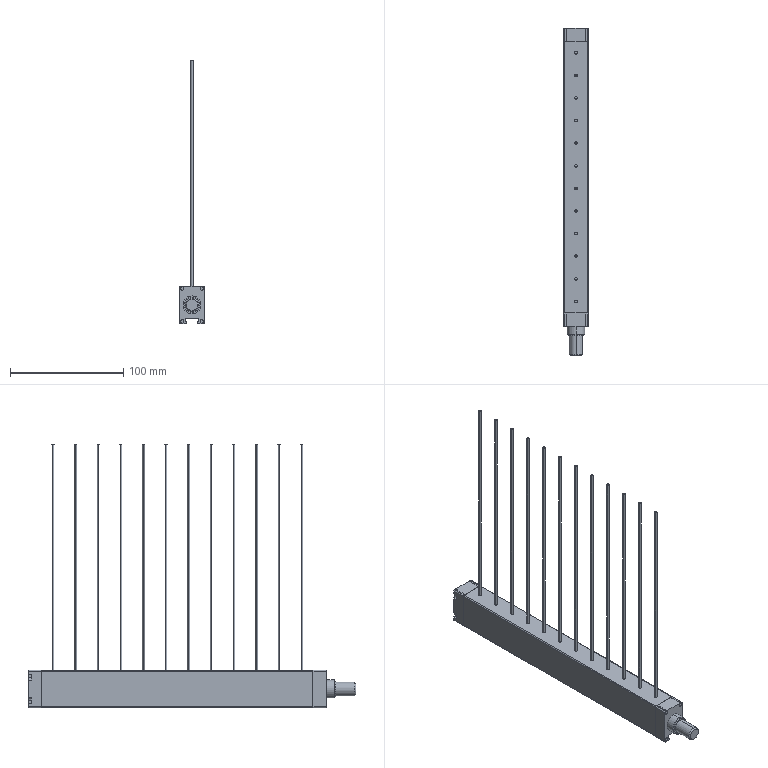Part | SolidWorks | features ICE 3, Extrusion 1, LPattern 1, MirrorPattern 1, Revolution 1 | 1 solid | 139 faces | box 22 x 290 x 232.8 mm | volume 181561 mm3 | plane 75 | cylinder 62 | cone 2 | commonest cylinder face diameters 2 x32 3 x16 1.6 x4 4 x4 12 x2 14 x2